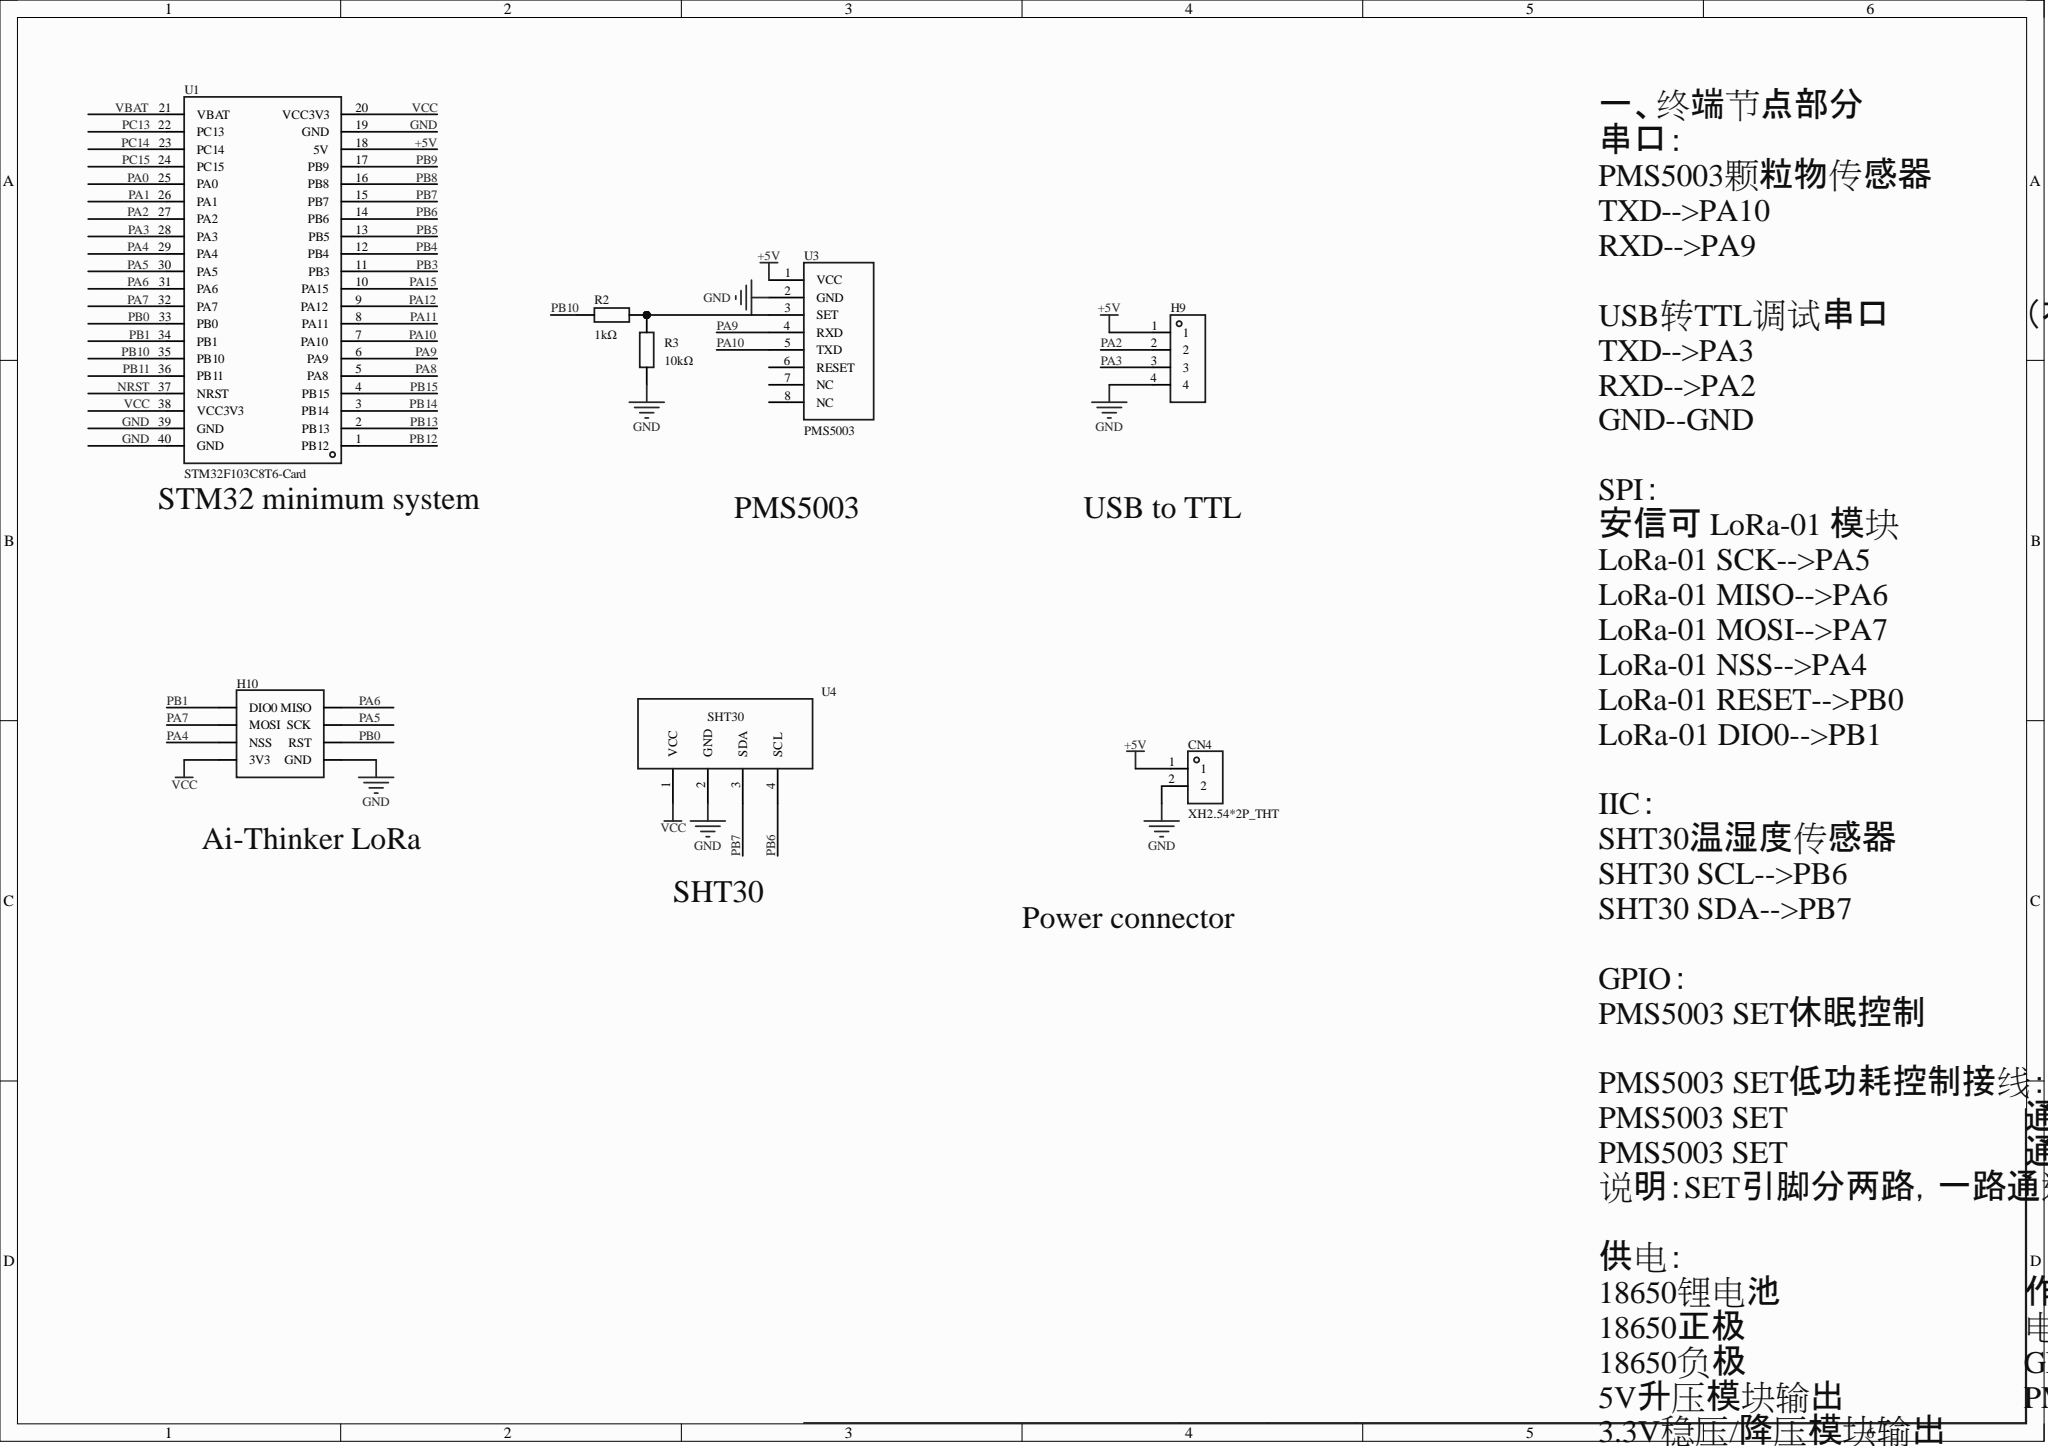Circuit board | Altium Designer | 8 parts | 17 nets
Bill of materials:
Comment,Description,Designator,Footprint,LibRef,Quantity
"XH2.54*2P_THT","","CN4","CONN-TH_2P-P2.50-XH2.54-2P","XH2.54*2P_直插","1"
"","","H9","HDR-TH_4P-P2.54-V-M","HDR-M_2.54_1x4P","1"
"","","H10","HDR-TH_8P-P2.54-V-F-R2-C4-S2.54-1","HDR-F_2.54_2x4","1"
"1kΩ","","R2","Res_1/8W","Res_AXIAL-1/8W","1"
"10kΩ","","R3","Res_1/8W","Res_AXIAL-1/8W","1"
"STM32F103C8T6-Card","","U1","CONN-TH_L53.3-W22.9_STM32F103C8T6-CARD","STM32F103C8T6-Card","1"
"PMS5003","","U3","1.25-LI-8P","PMS5003","1"
"","","U4","SHT30模块","SHT30","1"
Netlist (Protel format):
[
CN4
CONN-TH_2P-P2.50-XH2.54-2P
XH2.54*2P_THT



]
[
H9
HDR-TH_4P-P2.54-V-M




]
[
H10
HDR-TH_8P-P2.54-V-F-R2-C4-S2.54-1




]
[
R2
Res_1/8W
1kΩ



]
[
R3
Res_1/8W
10kΩ



]
[
U1
CONN-TH_L53.3-W22.9_STM32F103C8T6-CARD
STM32F103C8T6-Card



]
[
U3
1.25-LI-8P
PMS5003



]
[
U4
SHT30模块




]
(
VCC
H10-7
U1-20
U1-38
U4-1
)
(
PB10
R2-1
U1-35
)
(
PB7
U1-15
U4-3
)
(
PB6
U1-14
U4-4
)
(
PB1
H10-1
U1-34
)
(
PB0
H10-6
U1-33
)
(
PA10
U1-7
U3-5
)
(
PA9
U1-6
U3-4
)
(
PA7
H10-3
U1-32
)
(
PA6
H10-2
U1-31
)
(
PA5
H10-4
U1-30
)
(
PA4
H10-5
U1-29
)
(
PA3
H9-3
U1-28
)
(
PA2
H9-2
U1-27
)
(
NetR2_2
R2-2
R3-2
U3-3
)
(
GND
CN4-2
H9-4
H10-8
R3-1
U1-19
U1-39
U1-40
U3-2
U4-2
)
(
+5V
CN4-1
H9-1
U1-18
U3-1
)